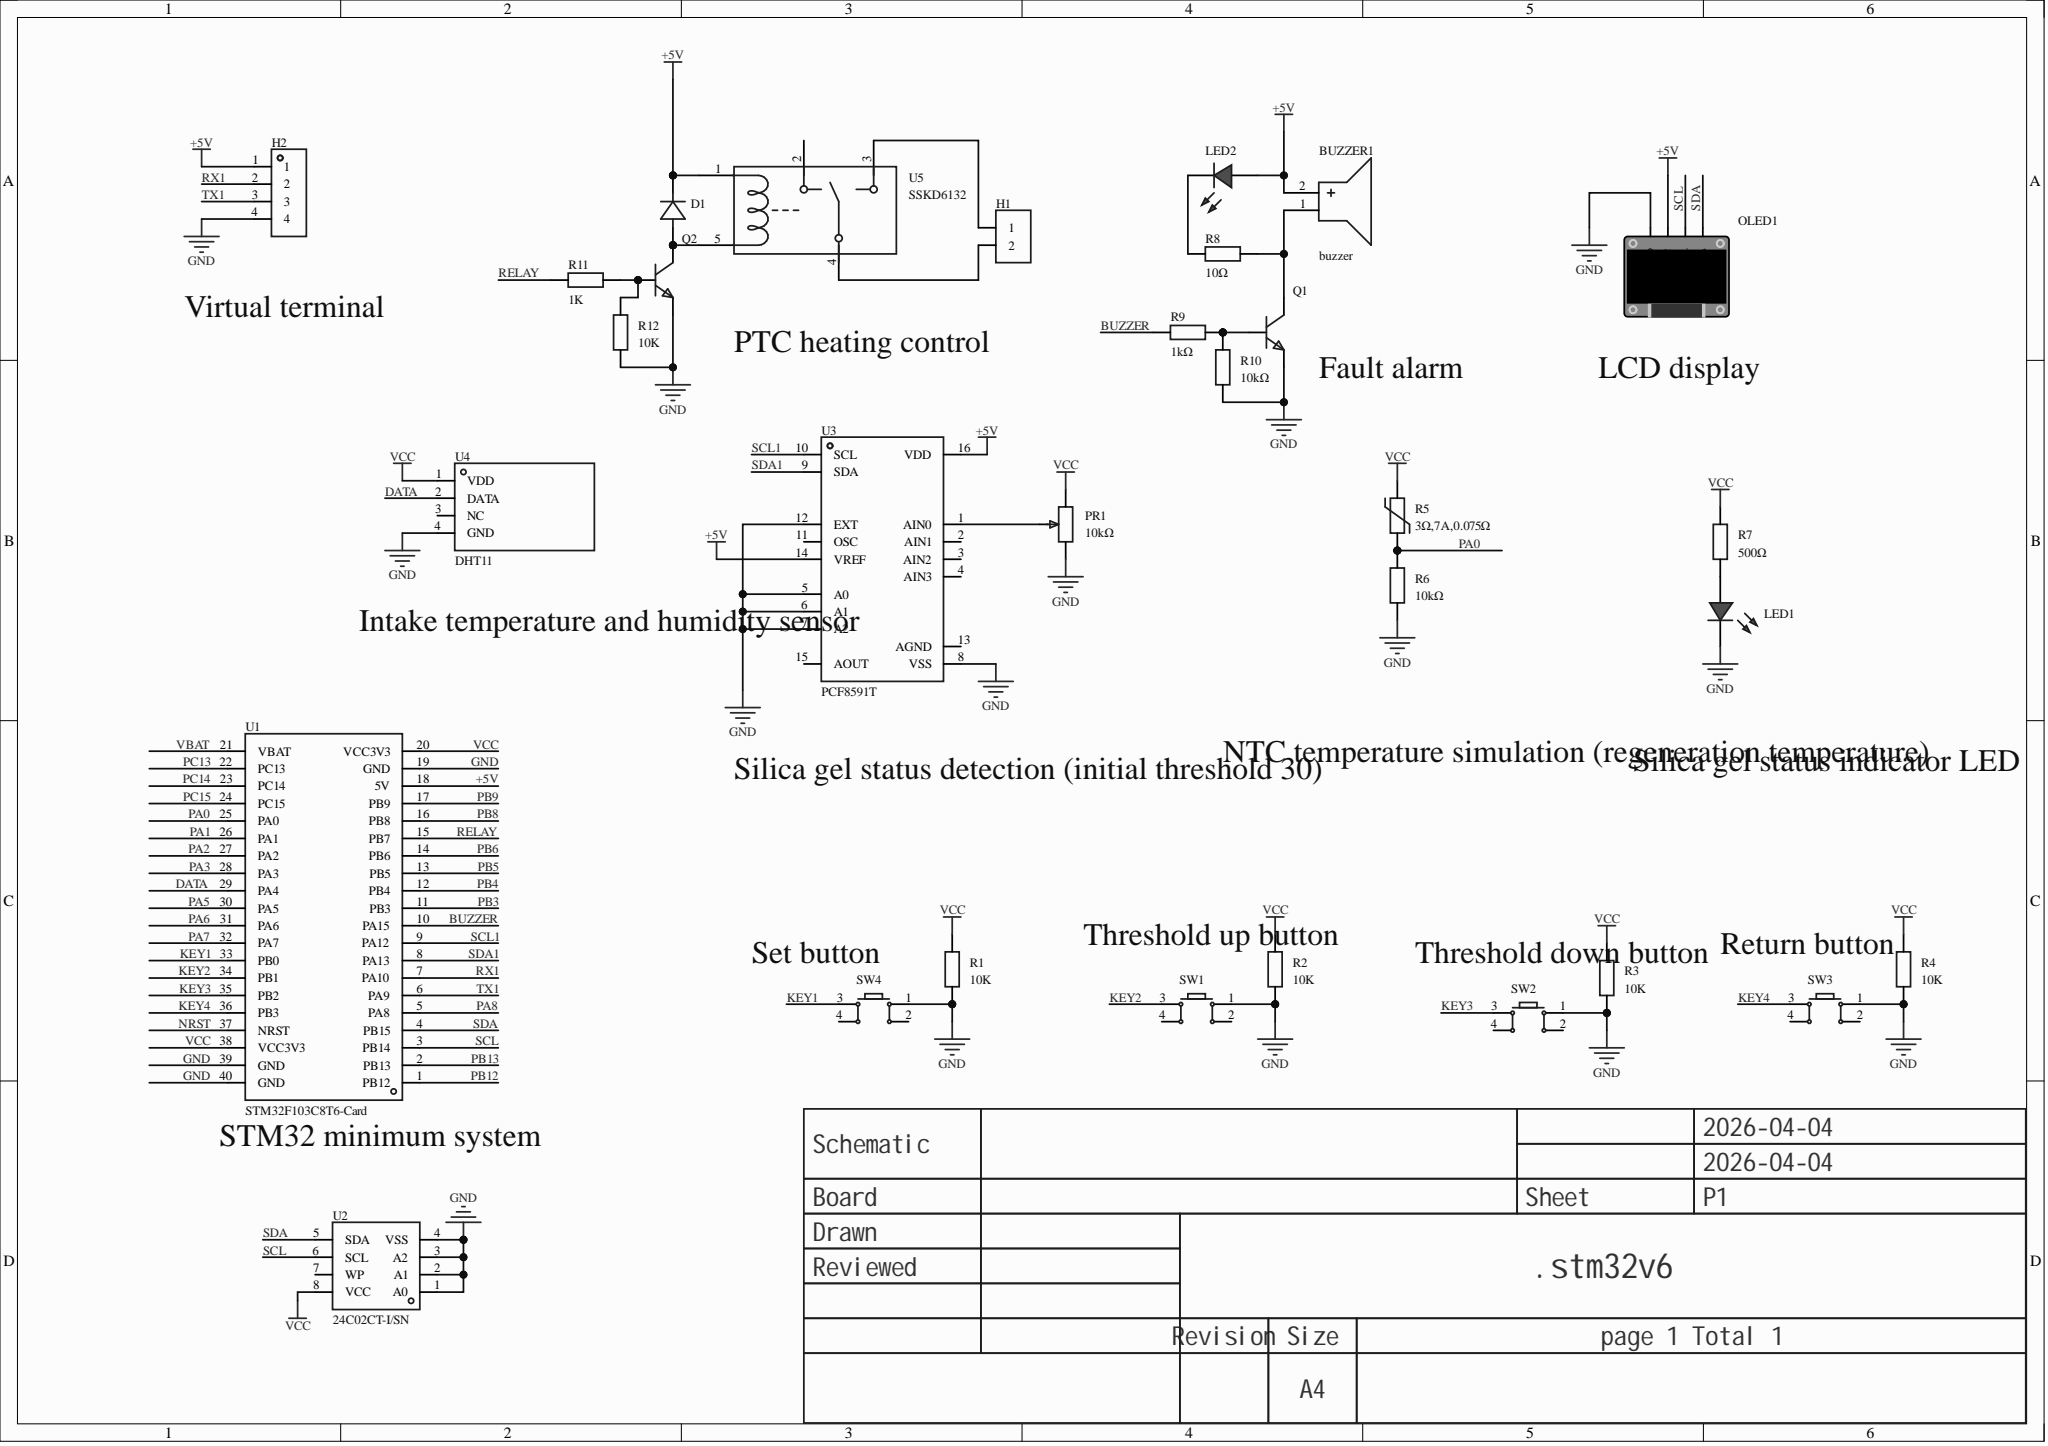Circuit board | Altium Designer | 31 parts | 26 nets
Bill of materials:
Comment,Description,Designator,Footprint,LibRef,Quantity
"buzzer","","BUZZER1","BUZ-TH_BD12.0-P6.00-D0.9-RD","buzzer","1"
"","","D1","DO_1N4007","D_1N4007A","1"
"","","H1","HDR-TH_2P-P2.54-V-F","HDR-F_2.54_1x2P","1"
"","","H2","HDR-TH_4P-P2.54-V-F","HDR-F_2.54_1x4P","1"
"","","LED1, LED2","LED_TH-3mm","LED_TH-R_3mm","2"
"","","OLED1","0.96OLED_4P","0.96OLED模块_4P","1"
"10kΩ","","PR1","R_3296","R_3296","1"
"","","Q1, Q2","S8050_TO_92","S8050_TO_NPN","2"
"10K","","R1, R2, R3, R4, R12","R0603","Res_0603","5"
"3Ω,7A,0.075Ω","","R5","RES-TH_L16.5-W7.0-P7.50-D0.8-S6.2","3Ω,7A,0.075Ω","1"
"10kΩ","","R6, R10","Res_1/8W","Res_AXIAL-1/8W","2"
"500Ω","","R7","Res_1/8W","Res_AXIAL-1/8W","1"
"10Ω","","R8","Res_1/8W","Res_AXIAL-1/8W","1"
"1kΩ","","R9","Res_1/8W","Res_AXIAL-1/8W","1"
"1K","","R11","R0603","Res_0603","1"
"","","SW1, SW2, SW3, SW4","SW-TH_4P-L6.0-W6.0-P4.50-LS6.5","Key_TH_6x6x6","4"
"STM32F103C8T6-Card","","U1","CONN-TH_L53.3-W22.9_STM32F103C8T6-CARD","STM32F103C8T6-Card","1"
"24C02CT-I/SN","Interface type: I2C; storage capacity: 2Kbit; clock frequency (fc): 400kHz;","U2","SOIC-8_L4.9-W3.9-P1.27-LS6.0-BL","24C02CT-I/SN","1"
"PCF8591T","","U3","SOIC-16_L10.3-W7.5-P1.27-LS10.3-BL","PCF8591T","1"
"DHT11","New capacitive digital temperature and humidity sensor; old model discontinued; 16.1x12.6x5.8mm","U4","SENSOR-TH_DHT11","DHT11","1"
"SSKD6132","","U5","RELAY-TH_G2R-1","SSKD6132","1"
Netlist (Protel format):
[
BUZZER1
BUZ-TH_BD12.0-P6.00-D0.9-RD
buzzer



]
[
D1
DO_1N4007




]
[
H1
HDR-TH_2P-P2.54-V-F




]
[
H2
HDR-TH_4P-P2.54-V-F




]
[
LED1
LED_TH-3mm




]
[
LED2
LED_TH-3mm




]
[
OLED1
0.96OLED_4P




]
[
PR1
R_3296
10kΩ



]
[
Q1
S8050_TO_92




]
[
Q2
S8050_TO_92




]
[
R1
R0603
10K



]
[
R2
R0603
10K



]
[
R3
R0603
10K



]
[
R4
R0603
10K



]
[
R5
RES-TH_L16.5-W7.0-P7.50-D0.8-S6.2
3Ω,7A,0.075Ω



]
[
R6
Res_1/8W
10kΩ



]
[
R7
Res_1/8W
500Ω



]
[
R8
Res_1/8W
10Ω



]
[
R9
Res_1/8W
1kΩ



]
[
R10
Res_1/8W
10kΩ



]
[
R11
R0603
1K



]
[
R12
R0603
10K



]
[
SW1
SW-TH_4P-L6.0-W6.0-P4.50-LS6.5




]
[
SW2
SW-TH_4P-L6.0-W6.0-P4.50-LS6.5




]
[
SW3
SW-TH_4P-L6.0-W6.0-P4.50-LS6.5




]
[
SW4
SW-TH_4P-L6.0-W6.0-P4.50-LS6.5




]
[
U1
CONN-TH_L53.3-W22.9_STM32F103C8T6-CARD
STM32F103C8T6-Card



]
[
U2
SOIC-8_L4.9-W3.9-P1.27-LS6.0-BL
24C02CT-I/SN



]
[
U3
SOIC-16_L10.3-W7.5-P1.27-LS10.3-BL
PCF8591T



]
[
U4
SENSOR-TH_DHT11
DHT11



]
[
U5
RELAY-TH_G2R-1
SSKD6132



]
(
VCC
PR1-1
R1-2
R2-2
R3-2
R4-2
R5-2
R7-2
U1-20
U1-38
U2-8
U4-1
)
(
TX1
H2-3
U1-6
)
(
SDA1
U1-8
U3-9
)
(
SDA
OLED1-4
U1-4
U2-5
)
(
SCL1
U1-9
U3-10
)
(
SCL
OLED1-3
U1-3
U2-6
)
(
RX1
H2-2
U1-7
)
(
RELAY
R11-1
U1-15
)
(
PA0
R5-1
R6-2
U1-25
)
(
NetQ2_2
Q2-2
R11-2
R12-2
)
(
NetQ1_2
Q1-2
R9-2
R10-2
)
(
NetPR1_2
PR1-2
U3-1
)
(
NetLED2_2
LED2-2
R8-2
)
(
NetLED1_1
LED1-1
R7-1
)
(
NetH1_2
H1-2
U5-4
)
(
NetH1_1
H1-1
U5-3
)
(
NetD1_2
D1-2
Q2-3
U5-5
)
(
NetBUZZER1_1
BUZZER1-1
Q1-3
R8-1
)
(
KEY4
SW3-3
U1-36
)
(
KEY3
SW2-3
U1-35
)
(
KEY2
SW1-3
U1-34
)
(
KEY1
SW4-3
U1-33
)
(
GND
H2-4
LED1-2
OLED1-1
PR1-3
Q1-1
Q2-1
R1-1
R2-1
R3-1
R4-1
R6-1
R10-1
R12-1
SW1-1
SW2-1
SW3-1
SW4-1
U1-19
U1-39
U1-40
U2-1
U2-2
U2-3
U2-4
U3-5
U3-6
U3-7
U3-8
U3-12
U4-4
)
(
DATA
U1-29
U4-2
)
(
BUZZER
R9-1
U1-10
)
(
+5V
BUZZER1-2
D1-1
H2-1
LED2-1
OLED1-2
U1-18
U3-14
U3-16
U5-1
)